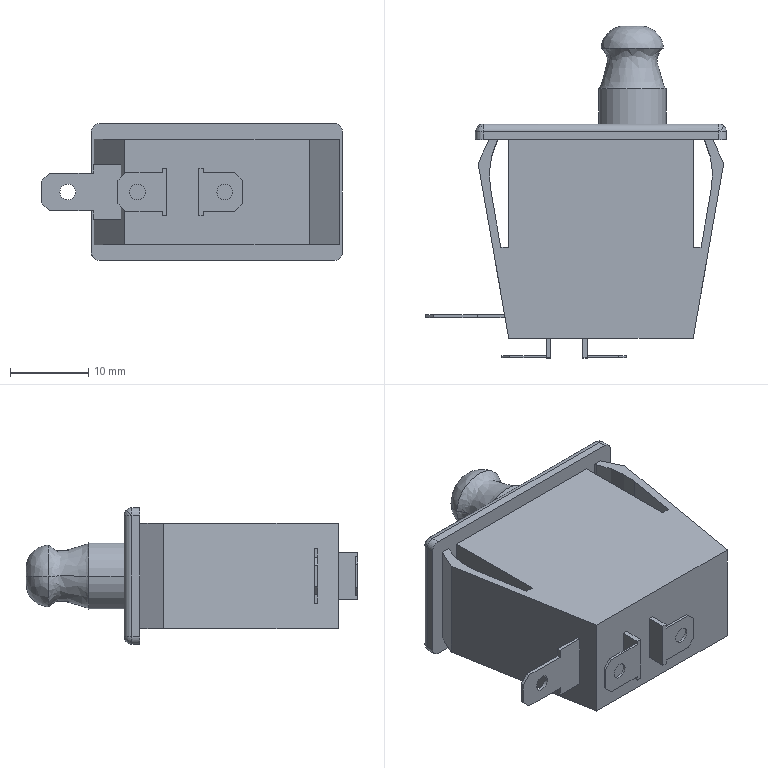Part | STEP file | NTAQZJ-AA-ANQUANKAIGUAN-061030.stp.STEP | 1 solid | 85 faces | box 38.35 x 42.3 x 17.4 mm | volume 10398 mm3 | plane 55 | cylinder 18 | sphere 8 | spline 4 | commonest cylinder face diameters 2 x14 8.6 x2 20 x2